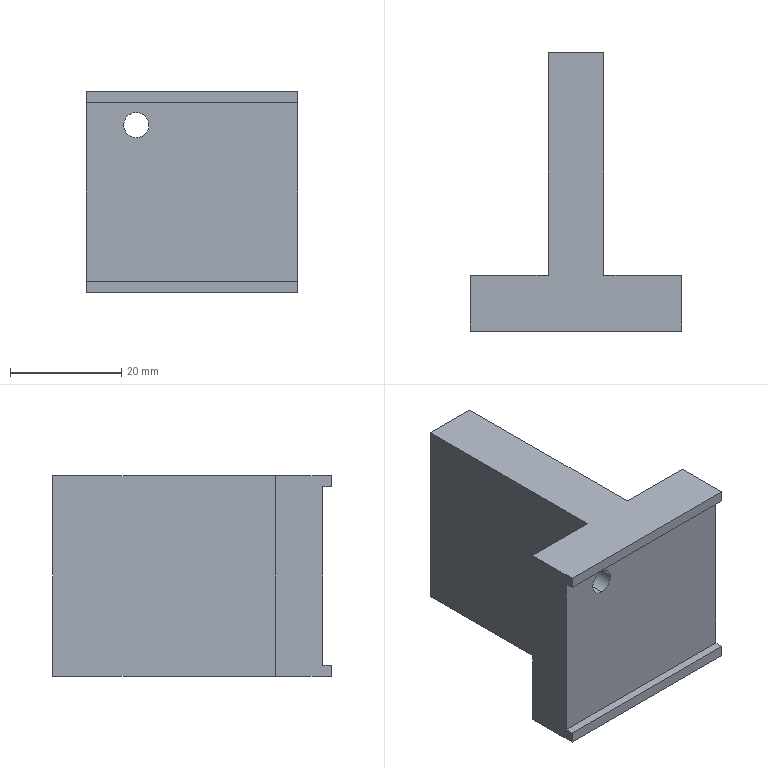Part | SolidWorks | features 3DProfileFeature 1, Extrusion 1, HoleWzd 1, ICE 1 | 1 solid | 19 faces | box 38 x 50 x 36 mm | volume 25963 mm3 | plane 15 | cylinder 4 | commonest cylinder face diameters 4.5 x2 8 x2
STEP:
#1=CARTESIAN_POINT('',(-10.,5.4,8.));
#2=VERTEX_POINT('',#1);
#3=CARTESIAN_POINT('',(-10.,5.4,16.));
#4=VERTEX_POINT('',#3);
#5=CARTESIAN_POINT('',(-10.,5.4,12.));
#6=DIRECTION('',(0.,1.,0.));
#7=DIRECTION('',(0.,0.,1.));
#8=AXIS2_PLACEMENT_3D('',#5,#6,#7);
#9=CIRCLE('',#8,4.);
#10=EDGE_CURVE('',#2,#4,#9,.T.);
#11=ORIENTED_EDGE('',*,*,#10,.F.);
#12=CARTESIAN_POINT('',(-10.,10.,8.));
#13=VERTEX_POINT('',#12);
#14=CARTESIAN_POINT('',(-10.,10.,8.));
#15=DIRECTION('',(0.,1.,0.));
#16=VECTOR('',#15,1000.);
#17=LINE('',#14,#16);
#18=EDGE_CURVE('',#2,#13,#17,.T.);
#19=ORIENTED_EDGE('',*,*,#18,.T.);
#20=CARTESIAN_POINT('',(-10.,10.,16.));
#21=VERTEX_POINT('',#20);
#22=CARTESIAN_POINT('',(-10.,10.,12.));
#23=DIRECTION('',(0.,1.,0.));
#24=DIRECTION('',(0.,0.,1.));
#25=AXIS2_PLACEMENT_3D('',#22,#23,#24);
#26=CIRCLE('',#25,4.);
#27=EDGE_CURVE('',#13,#21,#26,.T.);
#28=ORIENTED_EDGE('',*,*,#27,.T.);
#29=CARTESIAN_POINT('',(-10.,10.,16.));
#30=DIRECTION('',(0.,1.,0.));
#31=VECTOR('',#30,1000.);
#32=LINE('',#29,#31);
#33=EDGE_CURVE('',#4,#21,#32,.T.);
#34=ORIENTED_EDGE('',*,*,#33,.F.);
#35=EDGE_LOOP('',(#11,#19,#28,#34));
#36=FACE_OUTER_BOUND('',#35,.T.);
#37=CARTESIAN_POINT('',(-10.,10.,12.));
#38=DIRECTION('',(0.,1.,0.));
#39=DIRECTION('',(0.,0.,1.));
#40=AXIS2_PLACEMENT_3D('',#37,#38,#39);
#41=CYLINDRICAL_SURFACE('',#40,4.);
#42=ADVANCED_FACE('',(#36),#41,.F.);
#43=CARTESIAN_POINT('',(-10.,1.5,14.25));
#44=VERTEX_POINT('',#43);
#45=CARTESIAN_POINT('',(-10.,1.5,9.75));
#46=VERTEX_POINT('',#45);
#47=CARTESIAN_POINT('',(-10.,1.5,12.));
#48=DIRECTION('',(0.,-1.,0.));
#49=DIRECTION('',(1.,0.,0.));
#50=AXIS2_PLACEMENT_3D('',#47,#48,#49);
#51=CIRCLE('',#50,2.25);
#52=EDGE_CURVE('',#44,#46,#51,.T.);
#53=ORIENTED_EDGE('',*,*,#52,.T.);
#54=CARTESIAN_POINT('',(-10.,5.4,9.75));
#55=VERTEX_POINT('',#54);
#56=CARTESIAN_POINT('',(-10.,10.,9.75));
#57=DIRECTION('',(0.,1.,0.));
#58=VECTOR('',#57,1000.);
#59=LINE('',#56,#58);
#60=EDGE_CURVE('',#46,#55,#59,.T.);
#61=ORIENTED_EDGE('',*,*,#60,.T.);
#62=CARTESIAN_POINT('',(-10.,5.4,14.25));
#63=VERTEX_POINT('',#62);
#64=CARTESIAN_POINT('',(-10.,5.4,12.));
#65=DIRECTION('',(0.,1.,0.));
#66=DIRECTION('',(0.,0.,1.));
#67=AXIS2_PLACEMENT_3D('',#64,#65,#66);
#68=CIRCLE('',#67,2.25);
#69=EDGE_CURVE('',#55,#63,#68,.T.);
#70=ORIENTED_EDGE('',*,*,#69,.T.);
#71=CARTESIAN_POINT('',(-10.,10.,14.25));
#72=DIRECTION('',(0.,1.,0.));
#73=VECTOR('',#72,1000.);
#74=LINE('',#71,#73);
#75=EDGE_CURVE('',#44,#63,#74,.T.);
#76=ORIENTED_EDGE('',*,*,#75,.F.);
#77=EDGE_LOOP('',(#53,#61,#70,#76));
#78=FACE_OUTER_BOUND('',#77,.T.);
#79=CARTESIAN_POINT('',(-10.,10.,12.));
#80=DIRECTION('',(0.,1.,0.));
#81=DIRECTION('',(0.,0.,1.));
#82=AXIS2_PLACEMENT_3D('',#79,#80,#81);
#83=CYLINDRICAL_SURFACE('',#82,2.25);
#84=ADVANCED_FACE('',(#78),#83,.F.);
#85=CARTESIAN_POINT('',(19.,0.,-16.));
#86=VERTEX_POINT('',#85);
#87=CARTESIAN_POINT('',(19.,0.,-18.));
#88=VERTEX_POINT('',#87);
#89=CARTESIAN_POINT('',(19.,0.,18.));
#90=DIRECTION('',(0.,0.,-1.));
#91=VECTOR('',#90,1000.);
#92=LINE('',#89,#91);
#93=EDGE_CURVE('',#86,#88,#92,.T.);
#94=ORIENTED_EDGE('',*,*,#93,.F.);
#95=CARTESIAN_POINT('',(-19.,0.,-16.));
#96=VERTEX_POINT('',#95);
#97=CARTESIAN_POINT('',(-19.,0.,-16.));
#98=DIRECTION('',(1.,0.,0.));
#99=VECTOR('',#98,1000.);
#100=LINE('',#97,#99);
#101=EDGE_CURVE('',#96,#86,#100,.T.);
#102=ORIENTED_EDGE('',*,*,#101,.F.);
#103=CARTESIAN_POINT('',(-19.,0.,-18.));
#104=VERTEX_POINT('',#103);
#105=CARTESIAN_POINT('',(-19.,0.,18.));
#106=DIRECTION('',(0.,0.,-1.));
#107=VECTOR('',#106,1000.);
#108=LINE('',#105,#107);
#109=EDGE_CURVE('',#96,#104,#108,.T.);
#110=ORIENTED_EDGE('',*,*,#109,.T.);
#111=CARTESIAN_POINT('',(0.,0.,-18.));
#112=DIRECTION('',(1.,0.,0.));
#113=VECTOR('',#112,1000.);
#114=LINE('',#111,#113);
#115=EDGE_CURVE('',#104,#88,#114,.T.);
#116=ORIENTED_EDGE('',*,*,#115,.T.);
#117=EDGE_LOOP('',(#94,#102,#110,#116));
#118=FACE_OUTER_BOUND('',#117,.T.);
#119=CARTESIAN_POINT('',(0.,0.,18.));
#120=DIRECTION('',(0.,1.,0.));
#121=DIRECTION('',(-1.,0.,0.));
#122=AXIS2_PLACEMENT_3D('',#119,#120,#121);
#123=PLANE('',#122);
#124=ADVANCED_FACE('',(#118),#123,.F.);
#125=CARTESIAN_POINT('',(19.,1.5,-16.));
#126=VERTEX_POINT('',#125);
#127=CARTESIAN_POINT('',(19.,1.5,16.));
#128=VERTEX_POINT('',#127);
#129=CARTESIAN_POINT('',(19.,1.5,16.));
#130=DIRECTION('',(0.,0.,1.));
#131=VECTOR('',#130,1000.);
#132=LINE('',#129,#131);
#133=EDGE_CURVE('',#126,#128,#132,.T.);
#134=ORIENTED_EDGE('',*,*,#133,.F.);
#135=CARTESIAN_POINT('',(19.,1.5,-16.));
#136=DIRECTION('',(0.,-1.,0.));
#137=VECTOR('',#136,1000.);
#138=LINE('',#135,#137);
#139=EDGE_CURVE('',#126,#86,#138,.T.);
#140=ORIENTED_EDGE('',*,*,#139,.T.);
#141=ORIENTED_EDGE('',*,*,#93,.T.);
#142=CARTESIAN_POINT('',(19.,10.,-18.));
#143=VERTEX_POINT('',#142);
#144=CARTESIAN_POINT('',(19.,10.,-18.));
#145=DIRECTION('',(0.,1.,0.));
#146=VECTOR('',#145,1000.);
#147=LINE('',#144,#146);
#148=EDGE_CURVE('',#88,#143,#147,.T.);
#149=ORIENTED_EDGE('',*,*,#148,.T.);
#150=CARTESIAN_POINT('',(19.,10.,18.));
#151=VERTEX_POINT('',#150);
#152=CARTESIAN_POINT('',(19.,10.,18.));
#153=DIRECTION('',(0.,0.,-1.));
#154=VECTOR('',#153,1000.);
#155=LINE('',#152,#154);
#156=EDGE_CURVE('',#151,#143,#155,.T.);
#157=ORIENTED_EDGE('',*,*,#156,.F.);
#158=CARTESIAN_POINT('',(19.,0.,18.));
#159=VERTEX_POINT('',#158);
#160=CARTESIAN_POINT('',(19.,10.,18.));
#161=DIRECTION('',(0.,1.,0.));
#162=VECTOR('',#161,1000.);
#163=LINE('',#160,#162);
#164=EDGE_CURVE('',#159,#151,#163,.T.);
#165=ORIENTED_EDGE('',*,*,#164,.F.);
#166=CARTESIAN_POINT('',(19.,0.,16.));
#167=VERTEX_POINT('',#166);
#168=CARTESIAN_POINT('',(19.,0.,18.));
#169=DIRECTION('',(0.,0.,-1.));
#170=VECTOR('',#169,1000.);
#171=LINE('',#168,#170);
#172=EDGE_CURVE('',#159,#167,#171,.T.);
#173=ORIENTED_EDGE('',*,*,#172,.T.);
#174=CARTESIAN_POINT('',(19.,1.5,16.));
#175=DIRECTION('',(0.,-1.,0.));
#176=VECTOR('',#175,1000.);
#177=LINE('',#174,#176);
#178=EDGE_CURVE('',#128,#167,#177,.T.);
#179=ORIENTED_EDGE('',*,*,#178,.F.);
#180=EDGE_LOOP('',(#134,#140,#141,#149,#157,#165,#173,#179));
#181=FACE_OUTER_BOUND('',#180,.T.);
#182=CARTESIAN_POINT('',(19.,10.,18.));
#183=DIRECTION('',(-1.,0.,0.));
#184=DIRECTION('',(0.,-1.,0.));
#185=AXIS2_PLACEMENT_3D('',#182,#183,#184);
#186=PLANE('',#185);
#187=ADVANCED_FACE('',(#181),#186,.F.);
#188=CARTESIAN_POINT('',(5.,10.,-18.));
#189=VERTEX_POINT('',#188);
#190=CARTESIAN_POINT('',(5.,10.,-18.));
#191=DIRECTION('',(-1.,0.,0.));
#192=VECTOR('',#191,1000.);
#193=LINE('',#190,#192);
#194=EDGE_CURVE('',#143,#189,#193,.T.);
#195=ORIENTED_EDGE('',*,*,#194,.T.);
#196=CARTESIAN_POINT('',(5.,10.,18.));
#197=VERTEX_POINT('',#196);
#198=CARTESIAN_POINT('',(5.,10.,18.));
#199=DIRECTION('',(0.,0.,-1.));
#200=VECTOR('',#199,1000.);
#201=LINE('',#198,#200);
#202=EDGE_CURVE('',#197,#189,#201,.T.);
#203=ORIENTED_EDGE('',*,*,#202,.F.);
#204=CARTESIAN_POINT('',(5.,10.,18.));
#205=DIRECTION('',(-1.,0.,0.));
#206=VECTOR('',#205,1000.);
#207=LINE('',#204,#206);
#208=EDGE_CURVE('',#151,#197,#207,.T.);
#209=ORIENTED_EDGE('',*,*,#208,.F.);
#210=ORIENTED_EDGE('',*,*,#156,.T.);
#211=EDGE_LOOP('',(#195,#203,#209,#210));
#212=FACE_OUTER_BOUND('',#211,.T.);
#213=CARTESIAN_POINT('',(5.,10.,18.));
#214=DIRECTION('',(0.,-1.,0.));
#215=DIRECTION('',(1.,0.,0.));
#216=AXIS2_PLACEMENT_3D('',#213,#214,#215);
#217=PLANE('',#216);
#218=ADVANCED_FACE('',(#212),#217,.F.);
#219=CARTESIAN_POINT('',(5.,50.,-18.));
#220=VERTEX_POINT('',#219);
#221=CARTESIAN_POINT('',(5.,50.,-18.));
#222=DIRECTION('',(0.,1.,0.));
#223=VECTOR('',#222,1000.);
#224=LINE('',#221,#223);
#225=EDGE_CURVE('',#189,#220,#224,.T.);
#226=ORIENTED_EDGE('',*,*,#225,.T.);
#227=CARTESIAN_POINT('',(5.,50.,18.));
#228=VERTEX_POINT('',#227);
#229=CARTESIAN_POINT('',(5.,50.,18.));
#230=DIRECTION('',(0.,0.,-1.));
#231=VECTOR('',#230,1000.);
#232=LINE('',#229,#231);
#233=EDGE_CURVE('',#228,#220,#232,.T.);
#234=ORIENTED_EDGE('',*,*,#233,.F.);
#235=CARTESIAN_POINT('',(5.,50.,18.));
#236=DIRECTION('',(0.,1.,0.));
#237=VECTOR('',#236,1000.);
#238=LINE('',#235,#237);
#239=EDGE_CURVE('',#197,#228,#238,.T.);
#240=ORIENTED_EDGE('',*,*,#239,.F.);
#241=ORIENTED_EDGE('',*,*,#202,.T.);
#242=EDGE_LOOP('',(#226,#234,#240,#241));
#243=FACE_OUTER_BOUND('',#242,.T.);
#244=CARTESIAN_POINT('',(5.,50.,18.));
#245=DIRECTION('',(-1.,0.,0.));
#246=DIRECTION('',(0.,-1.,0.));
#247=AXIS2_PLACEMENT_3D('',#244,#245,#246);
#248=PLANE('',#247);
#249=ADVANCED_FACE('',(#243),#248,.F.);
#250=CARTESIAN_POINT('',(-5.,50.,-18.));
#251=VERTEX_POINT('',#250);
#252=CARTESIAN_POINT('',(-5.,50.,-18.));
#253=DIRECTION('',(-1.,0.,0.));
#254=VECTOR('',#253,1000.);
#255=LINE('',#252,#254);
#256=EDGE_CURVE('',#220,#251,#255,.T.);
#257=ORIENTED_EDGE('',*,*,#256,.T.);
#258=CARTESIAN_POINT('',(-5.,50.,18.));
#259=VERTEX_POINT('',#258);
#260=CARTESIAN_POINT('',(-5.,50.,18.));
#261=DIRECTION('',(0.,0.,-1.));
#262=VECTOR('',#261,1000.);
#263=LINE('',#260,#262);
#264=EDGE_CURVE('',#259,#251,#263,.T.);
#265=ORIENTED_EDGE('',*,*,#264,.F.);
#266=CARTESIAN_POINT('',(-5.,50.,18.));
#267=DIRECTION('',(-1.,0.,0.));
#268=VECTOR('',#267,1000.);
#269=LINE('',#266,#268);
#270=EDGE_CURVE('',#228,#259,#269,.T.);
#271=ORIENTED_EDGE('',*,*,#270,.F.);
#272=ORIENTED_EDGE('',*,*,#233,.T.);
#273=EDGE_LOOP('',(#257,#265,#271,#272));
#274=FACE_OUTER_BOUND('',#273,.T.);
#275=CARTESIAN_POINT('',(-5.,50.,18.));
#276=DIRECTION('',(0.,-1.,0.));
#277=DIRECTION('',(0.,0.,-1.));
#278=AXIS2_PLACEMENT_3D('',#275,#276,#277);
#279=PLANE('',#278);
#280=ADVANCED_FACE('',(#274),#279,.F.);
#281=CARTESIAN_POINT('',(-5.,10.,-18.));
#282=VERTEX_POINT('',#281);
#283=CARTESIAN_POINT('',(-5.,10.,-18.));
#284=DIRECTION('',(0.,-1.,0.));
#285=VECTOR('',#284,1000.);
#286=LINE('',#283,#285);
#287=EDGE_CURVE('',#251,#282,#286,.T.);
#288=ORIENTED_EDGE('',*,*,#287,.T.);
#289=CARTESIAN_POINT('',(-5.,10.,18.));
#290=VERTEX_POINT('',#289);
#291=CARTESIAN_POINT('',(-5.,10.,18.));
#292=DIRECTION('',(0.,0.,-1.));
#293=VECTOR('',#292,1000.);
#294=LINE('',#291,#293);
#295=EDGE_CURVE('',#290,#282,#294,.T.);
#296=ORIENTED_EDGE('',*,*,#295,.F.);
#297=CARTESIAN_POINT('',(-5.,10.,18.));
#298=DIRECTION('',(0.,-1.,0.));
#299=VECTOR('',#298,1000.);
#300=LINE('',#297,#299);
#301=EDGE_CURVE('',#259,#290,#300,.T.);
#302=ORIENTED_EDGE('',*,*,#301,.F.);
#303=ORIENTED_EDGE('',*,*,#264,.T.);
#304=EDGE_LOOP('',(#288,#296,#302,#303));
#305=FACE_OUTER_BOUND('',#304,.T.);
#306=CARTESIAN_POINT('',(-5.,10.,18.));
#307=DIRECTION('',(1.,0.,0.));
#308=DIRECTION('',(0.,0.,-1.));
#309=AXIS2_PLACEMENT_3D('',#306,#307,#308);
#310=PLANE('',#309);
#311=ADVANCED_FACE('',(#305),#310,.F.);
#312=CARTESIAN_POINT('',(-10.,10.,12.));
#313=DIRECTION('',(0.,1.,0.));
#314=DIRECTION('',(0.,0.,1.));
#315=AXIS2_PLACEMENT_3D('',#312,#313,#314);
#316=CIRCLE('',#315,4.);
#317=EDGE_CURVE('',#21,#13,#316,.T.);
#318=ORIENTED_EDGE('',*,*,#317,.F.);
#319=ORIENTED_EDGE('',*,*,#27,.F.);
#320=EDGE_LOOP('',(#318,#319));
#321=FACE_BOUND('',#320,.T.);
#322=CARTESIAN_POINT('',(-19.,10.,-18.));
#323=VERTEX_POINT('',#322);
#324=CARTESIAN_POINT('',(-19.,10.,-18.));
#325=DIRECTION('',(-1.,0.,0.));
#326=VECTOR('',#325,1000.);
#327=LINE('',#324,#326);
#328=EDGE_CURVE('',#282,#323,#327,.T.);
#329=ORIENTED_EDGE('',*,*,#328,.T.);
#330=CARTESIAN_POINT('',(-19.,10.,18.));
#331=VERTEX_POINT('',#330);
#332=CARTESIAN_POINT('',(-19.,10.,18.));
#333=DIRECTION('',(0.,0.,-1.));
#334=VECTOR('',#333,1000.);
#335=LINE('',#332,#334);
#336=EDGE_CURVE('',#331,#323,#335,.T.);
#337=ORIENTED_EDGE('',*,*,#336,.F.);
#338=CARTESIAN_POINT('',(-19.,10.,18.));
#339=DIRECTION('',(-1.,0.,0.));
#340=VECTOR('',#339,1000.);
#341=LINE('',#338,#340);
#342=EDGE_CURVE('',#290,#331,#341,.T.);
#343=ORIENTED_EDGE('',*,*,#342,.F.);
#344=ORIENTED_EDGE('',*,*,#295,.T.);
#345=EDGE_LOOP('',(#329,#337,#343,#344));
#346=FACE_OUTER_BOUND('',#345,.T.);
#347=CARTESIAN_POINT('',(-19.,10.,18.));
#348=DIRECTION('',(0.,-1.,0.));
#349=DIRECTION('',(0.,0.,-1.));
#350=AXIS2_PLACEMENT_3D('',#347,#348,#349);
#351=PLANE('',#350);
#352=ADVANCED_FACE('',(#321,#346),#351,.F.);
#353=ORIENTED_EDGE('',*,*,#109,.F.);
#354=CARTESIAN_POINT('',(-19.,1.5,-16.));
#355=VERTEX_POINT('',#354);
#356=CARTESIAN_POINT('',(-19.,1.5,-16.));
#357=DIRECTION('',(0.,-1.,0.));
#358=VECTOR('',#357,1000.);
#359=LINE('',#356,#358);
#360=EDGE_CURVE('',#355,#96,#359,.T.);
#361=ORIENTED_EDGE('',*,*,#360,.F.);
#362=CARTESIAN_POINT('',(-19.,1.5,16.));
#363=VERTEX_POINT('',#362);
#364=CARTESIAN_POINT('',(-19.,1.5,16.));
#365=DIRECTION('',(0.,0.,-1.));
#366=VECTOR('',#365,1000.);
#367=LINE('',#364,#366);
#368=EDGE_CURVE('',#363,#355,#367,.T.);
#369=ORIENTED_EDGE('',*,*,#368,.F.);
#370=CARTESIAN_POINT('',(-19.,0.,16.));
#371=VERTEX_POINT('',#370);
#372=CARTESIAN_POINT('',(-19.,1.5,16.));
#373=DIRECTION('',(0.,-1.,0.));
#374=VECTOR('',#373,1000.);
#375=LINE('',#372,#374);
#376=EDGE_CURVE('',#363,#371,#375,.T.);
#377=ORIENTED_EDGE('',*,*,#376,.T.);
#378=CARTESIAN_POINT('',(-19.,0.,18.));
#379=VERTEX_POINT('',#378);
#380=CARTESIAN_POINT('',(-19.,0.,18.));
#381=DIRECTION('',(0.,0.,-1.));
#382=VECTOR('',#381,1000.);
#383=LINE('',#380,#382);
#384=EDGE_CURVE('',#379,#371,#383,.T.);
#385=ORIENTED_EDGE('',*,*,#384,.F.);
#386=CARTESIAN_POINT('',(-19.,0.,18.));
#387=DIRECTION('',(0.,-1.,0.));
#388=VECTOR('',#387,1000.);
#389=LINE('',#386,#388);
#390=EDGE_CURVE('',#331,#379,#389,.T.);
#391=ORIENTED_EDGE('',*,*,#390,.F.);
#392=ORIENTED_EDGE('',*,*,#336,.T.);
#393=CARTESIAN_POINT('',(-19.,0.,-18.));
#394=DIRECTION('',(0.,-1.,0.));
#395=VECTOR('',#394,1000.);
#396=LINE('',#393,#395);
#397=EDGE_CURVE('',#323,#104,#396,.T.);
#398=ORIENTED_EDGE('',*,*,#397,.T.);
#399=EDGE_LOOP('',(#353,#361,#369,#377,#385,#391,#392,#398));
#400=FACE_OUTER_BOUND('',#399,.T.);
#401=CARTESIAN_POINT('',(-19.,0.,18.));
#402=DIRECTION('',(1.,0.,0.));
#403=DIRECTION('',(0.,1.,0.));
#404=AXIS2_PLACEMENT_3D('',#401,#402,#403);
#405=PLANE('',#404);
#406=ADVANCED_FACE('',(#400),#405,.F.);
#407=ORIENTED_EDGE('',*,*,#384,.T.);
#408=CARTESIAN_POINT('',(-19.,0.,16.));
#409=DIRECTION('',(-1.,0.,0.));
#410=VECTOR('',#409,1000.);
#411=LINE('',#408,#410);
#412=EDGE_CURVE('',#167,#371,#411,.T.);
#413=ORIENTED_EDGE('',*,*,#412,.F.);
#414=ORIENTED_EDGE('',*,*,#172,.F.);
#415=CARTESIAN_POINT('',(19.,0.,18.));
#416=DIRECTION('',(1.,0.,0.));
#417=VECTOR('',#416,1000.);
#418=LINE('',#415,#417);
#419=EDGE_CURVE('',#379,#159,#418,.T.);
#420=ORIENTED_EDGE('',*,*,#419,.F.);
#421=EDGE_LOOP('',(#407,#413,#414,#420));
#422=FACE_OUTER_BOUND('',#421,.T.);
#423=CARTESIAN_POINT('',(0.,0.,18.));
#424=DIRECTION('',(0.,1.,0.));
#425=DIRECTION('',(-1.,0.,0.));
#426=AXIS2_PLACEMENT_3D('',#423,#424,#425);
#427=PLANE('',#426);
#428=ADVANCED_FACE('',(#422),#427,.F.);
#429=ORIENTED_EDGE('',*,*,#419,.T.);
#430=ORIENTED_EDGE('',*,*,#164,.T.);
#431=ORIENTED_EDGE('',*,*,#208,.T.);
#432=ORIENTED_EDGE('',*,*,#239,.T.);
#433=ORIENTED_EDGE('',*,*,#270,.T.);
#434=ORIENTED_EDGE('',*,*,#301,.T.);
#435=ORIENTED_EDGE('',*,*,#342,.T.);
#436=ORIENTED_EDGE('',*,*,#390,.T.);
#437=EDGE_LOOP('',(#429,#430,#431,#432,#433,#434,#435,#436));
#438=FACE_OUTER_BOUND('',#437,.T.);
#439=CARTESIAN_POINT('',(0.,0.,18.));
#440=DIRECTION('',(0.,0.,-1.));
#441=DIRECTION('',(-1.,0.,0.));
#442=AXIS2_PLACEMENT_3D('',#439,#440,#441);
#443=PLANE('',#442);
#444=ADVANCED_FACE('',(#438),#443,.F.);
#445=ORIENTED_EDGE('',*,*,#148,.F.);
#446=ORIENTED_EDGE('',*,*,#115,.F.);
#447=ORIENTED_EDGE('',*,*,#397,.F.);
#448=ORIENTED_EDGE('',*,*,#328,.F.);
#449=ORIENTED_EDGE('',*,*,#287,.F.);
#450=ORIENTED_EDGE('',*,*,#256,.F.);
#451=ORIENTED_EDGE('',*,*,#225,.F.);
#452=ORIENTED_EDGE('',*,*,#194,.F.);
#453=EDGE_LOOP('',(#445,#446,#447,#448,#449,#450,#451,#452));
#454=FACE_OUTER_BOUND('',#453,.T.);
#455=CARTESIAN_POINT('',(0.,0.,-18.));
#456=DIRECTION('',(0.,0.,-1.));
#457=DIRECTION('',(-1.,0.,0.));
#458=AXIS2_PLACEMENT_3D('',#455,#456,#457);
#459=PLANE('',#458);
#460=ADVANCED_FACE('',(#454),#459,.T.);
#461=ORIENTED_EDGE('',*,*,#101,.T.);
#462=ORIENTED_EDGE('',*,*,#139,.F.);
#463=CARTESIAN_POINT('',(-19.,1.5,-16.));
#464=DIRECTION('',(1.,0.,0.));
#465=VECTOR('',#464,1000.);
#466=LINE('',#463,#465);
#467=EDGE_CURVE('',#355,#126,#466,.T.);
#468=ORIENTED_EDGE('',*,*,#467,.F.);
#469=ORIENTED_EDGE('',*,*,#360,.T.);
#470=EDGE_LOOP('',(#461,#462,#468,#469));
#471=FACE_OUTER_BOUND('',#470,.T.);
#472=CARTESIAN_POINT('',(-19.,1.5,-16.));
#473=DIRECTION('',(0.,0.,-1.));
#474=DIRECTION('',(-1.,0.,0.));
#475=AXIS2_PLACEMENT_3D('',#472,#473,#474);
#476=PLANE('',#475);
#477=ADVANCED_FACE('',(#471),#476,.F.);
#478=ORIENTED_EDGE('',*,*,#412,.T.);
#479=ORIENTED_EDGE('',*,*,#376,.F.);
#480=CARTESIAN_POINT('',(-19.,1.5,16.));
#481=DIRECTION('',(-1.,0.,0.));
#482=VECTOR('',#481,1000.);
#483=LINE('',#480,#482);
#484=EDGE_CURVE('',#128,#363,#483,.T.);
#485=ORIENTED_EDGE('',*,*,#484,.F.);
#486=ORIENTED_EDGE('',*,*,#178,.T.);
#487=EDGE_LOOP('',(#478,#479,#485,#486));
#488=FACE_OUTER_BOUND('',#487,.T.);
#489=CARTESIAN_POINT('',(-19.,1.5,16.));
#490=DIRECTION('',(0.,0.,1.));
#491=DIRECTION('',(1.,0.,0.));
#492=AXIS2_PLACEMENT_3D('',#489,#490,#491);
#493=PLANE('',#492);
#494=ADVANCED_FACE('',(#488),#493,.F.);
#495=ORIENTED_EDGE('',*,*,#52,.F.);
#496=CARTESIAN_POINT('',(-10.,1.5,12.));
#497=DIRECTION('',(0.,-1.,0.));
#498=DIRECTION('',(1.,0.,0.));
#499=AXIS2_PLACEMENT_3D('',#496,#497,#498);
#500=CIRCLE('',#499,2.25);
#501=EDGE_CURVE('',#46,#44,#500,.T.);
#502=ORIENTED_EDGE('',*,*,#501,.F.);
#503=EDGE_LOOP('',(#495,#502));
#504=FACE_BOUND('',#503,.T.);
#505=ORIENTED_EDGE('',*,*,#133,.T.);
#506=ORIENTED_EDGE('',*,*,#484,.T.);
#507=ORIENTED_EDGE('',*,*,#368,.T.);
#508=ORIENTED_EDGE('',*,*,#467,.T.);
#509=EDGE_LOOP('',(#505,#506,#507,#508));
#510=FACE_OUTER_BOUND('',#509,.T.);
#511=CARTESIAN_POINT('',(0.,1.5,0.));
#512=DIRECTION('',(0.,-1.,0.));
#513=DIRECTION('',(1.,0.,0.));
#514=AXIS2_PLACEMENT_3D('',#511,#512,#513);
#515=PLANE('',#514);
#516=ADVANCED_FACE('',(#504,#510),#515,.T.);
#517=ORIENTED_EDGE('',*,*,#60,.F.);
#518=ORIENTED_EDGE('',*,*,#501,.T.);
#519=ORIENTED_EDGE('',*,*,#75,.T.);
#520=CARTESIAN_POINT('',(-10.,5.4,12.));
#521=DIRECTION('',(0.,1.,0.));
#522=DIRECTION('',(0.,0.,1.));
#523=AXIS2_PLACEMENT_3D('',#520,#521,#522);
#524=CIRCLE('',#523,2.25);
#525=EDGE_CURVE('',#63,#55,#524,.T.);
#526=ORIENTED_EDGE('',*,*,#525,.T.);
#527=EDGE_LOOP('',(#517,#518,#519,#526));
#528=FACE_OUTER_BOUND('',#527,.T.);
#529=CARTESIAN_POINT('',(-10.,10.,12.));
#530=DIRECTION('',(0.,1.,0.));
#531=DIRECTION('',(0.,0.,1.));
#532=AXIS2_PLACEMENT_3D('',#529,#530,#531);
#533=CYLINDRICAL_SURFACE('',#532,2.25);
#534=ADVANCED_FACE('',(#528),#533,.F.);
#535=ORIENTED_EDGE('',*,*,#525,.F.);
#536=ORIENTED_EDGE('',*,*,#69,.F.);
#537=EDGE_LOOP('',(#535,#536));
#538=FACE_BOUND('',#537,.T.);
#539=CARTESIAN_POINT('',(-10.,5.4,12.));
#540=DIRECTION('',(0.,1.,0.));
#541=DIRECTION('',(0.,0.,1.));
#542=AXIS2_PLACEMENT_3D('',#539,#540,#541);
#543=CIRCLE('',#542,4.);
#544=EDGE_CURVE('',#4,#2,#543,.T.);
#545=ORIENTED_EDGE('',*,*,#544,.T.);
#546=ORIENTED_EDGE('',*,*,#10,.T.);
#547=EDGE_LOOP('',(#545,#546));
#548=FACE_OUTER_BOUND('',#547,.T.);
#549=CARTESIAN_POINT('',(-7.75,5.4,12.));
#550=DIRECTION('',(0.,-1.,0.));
#551=DIRECTION('',(0.,0.,-1.));
#552=AXIS2_PLACEMENT_3D('',#549,#550,#551);
#553=PLANE('',#552);
#554=ADVANCED_FACE('',(#538,#548),#553,.F.);
#555=ORIENTED_EDGE('',*,*,#18,.F.);
#556=ORIENTED_EDGE('',*,*,#544,.F.);
#557=ORIENTED_EDGE('',*,*,#33,.T.);
#558=ORIENTED_EDGE('',*,*,#317,.T.);
#559=EDGE_LOOP('',(#555,#556,#557,#558));
#560=FACE_OUTER_BOUND('',#559,.T.);
#561=CARTESIAN_POINT('',(-10.,10.,12.));
#562=DIRECTION('',(0.,1.,0.));
#563=DIRECTION('',(0.,0.,1.));
#564=AXIS2_PLACEMENT_3D('',#561,#562,#563);
#565=CYLINDRICAL_SURFACE('',#564,4.);
#566=ADVANCED_FACE('',(#560),#565,.F.);
#567=CLOSED_SHELL('',(#42,#84,#124,#187,#218,#249,#280,#311,#352,#406,#428,#444,#460,#477,#494,#516,#534,#554,#566));
#568=MANIFOLD_SOLID_BREP('',#567);
#569=CARTESIAN_POINT('',(0.,0.,0.));
#570=DIRECTION('',(0.,0.,1.));
#571=DIRECTION('',(1.,0.,0.));
#572=AXIS2_PLACEMENT_3D('',#569,#570,#571);
#573=(LENGTH_UNIT()NAMED_UNIT(*)SI_UNIT(.MILLI.,.METRE.));
#574=UNCERTAINTY_MEASURE_WITH_UNIT(LENGTH_MEASURE(0.00001),#573,'','');
#575=(NAMED_UNIT(*)PLANE_ANGLE_UNIT()SI_UNIT($,.RADIAN.));
#576=(NAMED_UNIT(*)SI_UNIT($,.STERADIAN.)SOLID_ANGLE_UNIT());
#577=(GEOMETRIC_REPRESENTATION_CONTEXT(3)GLOBAL_UNCERTAINTY_ASSIGNED_CONTEXT((#574))GLOBAL_UNIT_ASSIGNED_CONTEXT((#573,#575,#576))REPRESENTATION_CONTEXT('',''));
#578=ADVANCED_BREP_SHAPE_REPRESENTATION('',(#568,#572),#577);